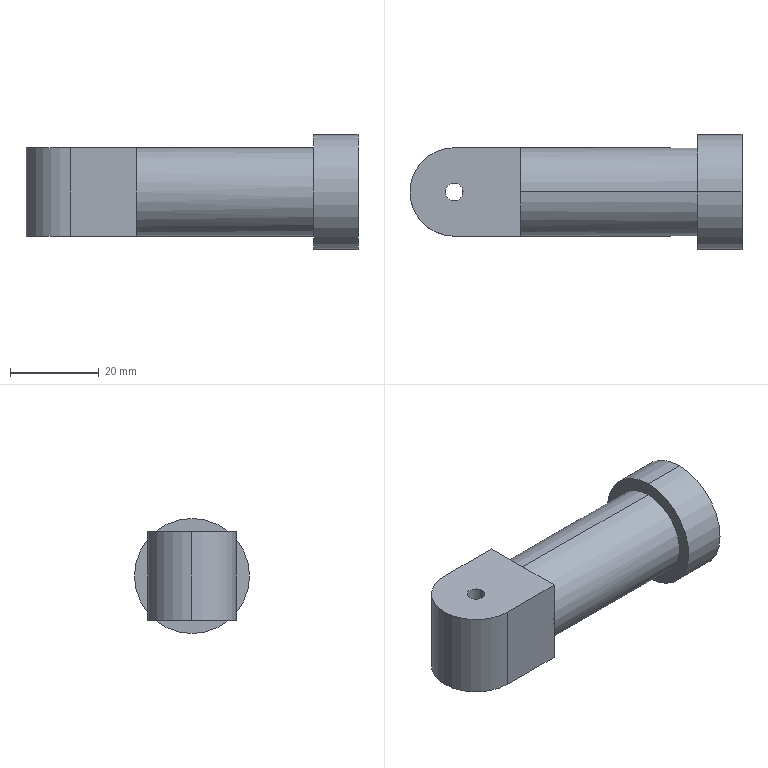Part | SolidWorks | features BaseBody 1 | 1 solid | 22 faces | box 75 x 26 x 26 mm | volume 24031 mm3 | cylinder 10 | plane 10 | cone 2 | commonest cylinder face diameters 20 x4 4 x2 16 x2 26 x2
STEP:
#1=CARTESIAN_POINT('',(15.081,-24.276,18.));
#2=VERTEX_POINT('',#1);
#3=CARTESIAN_POINT('',(15.081,-24.276,2.));
#4=VERTEX_POINT('',#3);
#5=CARTESIAN_POINT('',(15.081,-24.276,10.));
#6=DIRECTION('',(1.,0.,0.));
#7=DIRECTION('',(0.,0.,-1.));
#8=AXIS2_PLACEMENT_3D('',#5,#6,#7);
#9=CIRCLE('',#8,8.);
#10=EDGE_CURVE('',#2,#4,#9,.T.);
#11=ORIENTED_EDGE('',*,*,#10,.F.);
#12=CARTESIAN_POINT('',(27.081,-24.276,18.));
#13=VERTEX_POINT('',#12);
#14=CARTESIAN_POINT('',(27.081,-24.276,18.));
#15=DIRECTION('',(1.,0.,0.));
#16=VECTOR('',#15,1000.);
#17=LINE('',#14,#16);
#18=EDGE_CURVE('',#2,#13,#17,.T.);
#19=ORIENTED_EDGE('',*,*,#18,.T.);
#20=CARTESIAN_POINT('',(27.081,-24.276,2.));
#21=VERTEX_POINT('',#20);
#22=CARTESIAN_POINT('',(27.081,-24.276,10.));
#23=DIRECTION('',(1.,0.,0.));
#24=DIRECTION('',(0.,0.,-1.));
#25=AXIS2_PLACEMENT_3D('',#22,#23,#24);
#26=CIRCLE('',#25,8.);
#27=EDGE_CURVE('',#13,#21,#26,.T.);
#28=ORIENTED_EDGE('',*,*,#27,.T.);
#29=CARTESIAN_POINT('',(27.081,-24.276,2.));
#30=DIRECTION('',(1.,0.,0.));
#31=VECTOR('',#30,1000.);
#32=LINE('',#29,#31);
#33=EDGE_CURVE('',#4,#21,#32,.T.);
#34=ORIENTED_EDGE('',*,*,#33,.F.);
#35=EDGE_LOOP('',(#11,#19,#28,#34));
#36=FACE_OUTER_BOUND('',#35,.T.);
#37=CARTESIAN_POINT('',(27.081,-24.276,10.));
#38=DIRECTION('',(1.,0.,0.));
#39=DIRECTION('',(0.,0.,-1.));
#40=AXIS2_PLACEMENT_3D('',#37,#38,#39);
#41=CYLINDRICAL_SURFACE('',#40,8.);
#42=ADVANCED_FACE('',(#36),#41,.F.);
#43=CARTESIAN_POINT('',(10.274,-24.276,10.));
#44=VERTEX_POINT('',#43);
#45=CARTESIAN_POINT('',(15.081,-24.276,2.));
#46=DIRECTION('',(0.515,0.,-0.8572));
#47=VECTOR('',#46,1000.);
#48=LINE('',#45,#47);
#49=EDGE_CURVE('',#44,#4,#48,.T.);
#50=ORIENTED_EDGE('',*,*,#49,.F.);
#51=CARTESIAN_POINT('',(15.081,-24.276,18.));
#52=DIRECTION('',(0.515,0.,0.8572));
#53=VECTOR('',#52,1000.);
#54=LINE('',#51,#53);
#55=EDGE_CURVE('',#44,#2,#54,.T.);
#56=ORIENTED_EDGE('',*,*,#55,.T.);
#57=ORIENTED_EDGE('',*,*,#10,.T.);
#58=EDGE_LOOP('',(#50,#56,#57));
#59=FACE_OUTER_BOUND('',#58,.T.);
#60=CARTESIAN_POINT('',(15.081,-24.276,10.));
#61=DIRECTION('',(1.,0.,0.));
#62=DIRECTION('',(0.,0.,-1.));
#63=AXIS2_PLACEMENT_3D('',#60,#61,#62);
#64=CONICAL_SURFACE('',#63,8.,1.03);
#65=ADVANCED_FACE('',(#59),#64,.F.);
#66=CARTESIAN_POINT('',(17.081,-24.276,-3.));
#67=VERTEX_POINT('',#66);
#68=CARTESIAN_POINT('',(17.081,-24.276,23.));
#69=VERTEX_POINT('',#68);
#70=CARTESIAN_POINT('',(17.081,-24.276,10.));
#71=DIRECTION('',(1.,0.,0.));
#72=DIRECTION('',(0.,0.,-1.));
#73=AXIS2_PLACEMENT_3D('',#70,#71,#72);
#74=CIRCLE('',#73,13.);
#75=EDGE_CURVE('',#67,#69,#74,.T.);
#76=ORIENTED_EDGE('',*,*,#75,.T.);
#77=CARTESIAN_POINT('',(27.081,-24.276,23.));
#78=VERTEX_POINT('',#77);
#79=CARTESIAN_POINT('',(17.081,-24.276,23.));
#80=DIRECTION('',(1.,0.,0.));
#81=VECTOR('',#80,1000.);
#82=LINE('',#79,#81);
#83=EDGE_CURVE('',#69,#78,#82,.T.);
#84=ORIENTED_EDGE('',*,*,#83,.T.);
#85=CARTESIAN_POINT('',(27.081,-24.276,-3.));
#86=VERTEX_POINT('',#85);
#87=CARTESIAN_POINT('',(27.081,-24.276,10.));
#88=DIRECTION('',(1.,0.,0.));
#89=DIRECTION('',(0.,0.,-1.));
#90=AXIS2_PLACEMENT_3D('',#87,#88,#89);
#91=CIRCLE('',#90,13.);
#92=EDGE_CURVE('',#86,#78,#91,.T.);
#93=ORIENTED_EDGE('',*,*,#92,.F.);
#94=CARTESIAN_POINT('',(17.081,-24.276,-3.));
#95=DIRECTION('',(1.,0.,0.));
#96=VECTOR('',#95,1000.);
#97=LINE('',#94,#96);
#98=EDGE_CURVE('',#67,#86,#97,.T.);
#99=ORIENTED_EDGE('',*,*,#98,.F.);
#100=EDGE_LOOP('',(#76,#84,#93,#99));
#101=FACE_OUTER_BOUND('',#100,.T.);
#102=CARTESIAN_POINT('',(17.081,-24.276,10.));
#103=DIRECTION('',(1.,0.,0.));
#104=DIRECTION('',(0.,0.,-1.));
#105=AXIS2_PLACEMENT_3D('',#102,#103,#104);
#106=CYLINDRICAL_SURFACE('',#105,13.);
#107=ADVANCED_FACE('',(#101),#106,.T.);
#108=CARTESIAN_POINT('',(-39.919,-24.276,0.));
#109=VERTEX_POINT('',#108);
#110=CARTESIAN_POINT('',(-35.919,-24.276,0.));
#111=VERTEX_POINT('',#110);
#112=CARTESIAN_POINT('',(-37.919,-24.276,0.));
#113=DIRECTION('',(0.,0.,1.));
#114=DIRECTION('',(1.,0.,0.));
#115=AXIS2_PLACEMENT_3D('',#112,#113,#114);
#116=CIRCLE('',#115,2.);
#117=EDGE_CURVE('',#109,#111,#116,.T.);
#118=ORIENTED_EDGE('',*,*,#117,.F.);
#119=CARTESIAN_POINT('',(-39.919,-24.276,20.));
#120=VERTEX_POINT('',#119);
#121=CARTESIAN_POINT('',(-39.919,-24.276,20.));
#122=DIRECTION('',(0.,0.,1.));
#123=VECTOR('',#122,1000.);
#124=LINE('',#121,#123);
#125=EDGE_CURVE('',#109,#120,#124,.T.);
#126=ORIENTED_EDGE('',*,*,#125,.T.);
#127=CARTESIAN_POINT('',(-35.919,-24.276,20.));
#128=VERTEX_POINT('',#127);
#129=CARTESIAN_POINT('',(-37.919,-24.276,20.));
#130=DIRECTION('',(0.,0.,1.));
#131=DIRECTION('',(1.,0.,0.));
#132=AXIS2_PLACEMENT_3D('',#129,#130,#131);
#133=CIRCLE('',#132,2.);
#134=EDGE_CURVE('',#120,#128,#133,.T.);
#135=ORIENTED_EDGE('',*,*,#134,.T.);
#136=CARTESIAN_POINT('',(-35.919,-24.276,20.));
#137=DIRECTION('',(0.,0.,1.));
#138=VECTOR('',#137,1000.);
#139=LINE('',#136,#138);
#140=EDGE_CURVE('',#111,#128,#139,.T.);
#141=ORIENTED_EDGE('',*,*,#140,.F.);
#142=EDGE_LOOP('',(#118,#126,#135,#141));
#143=FACE_OUTER_BOUND('',#142,.T.);
#144=CARTESIAN_POINT('',(-37.919,-24.276,20.));
#145=DIRECTION('',(0.,0.,1.));
#146=DIRECTION('',(1.,0.,0.));
#147=AXIS2_PLACEMENT_3D('',#144,#145,#146);
#148=CYLINDRICAL_SURFACE('',#147,2.);
#149=ADVANCED_FACE('',(#143),#148,.F.);
#150=CARTESIAN_POINT('',(-47.919,-24.276,20.));
#151=VERTEX_POINT('',#150);
#152=CARTESIAN_POINT('',(-37.919,-34.276,20.));
#153=VERTEX_POINT('',#152);
#154=CARTESIAN_POINT('',(-37.919,-24.276,20.));
#155=DIRECTION('',(0.,0.,1.));
#156=DIRECTION('',(1.,0.,0.));
#157=AXIS2_PLACEMENT_3D('',#154,#155,#156);
#158=CIRCLE('',#157,10.);
#159=EDGE_CURVE('',#151,#153,#158,.T.);
#160=ORIENTED_EDGE('',*,*,#159,.F.);
#161=CARTESIAN_POINT('',(-47.919,-24.276,0.));
#162=VERTEX_POINT('',#161);
#163=CARTESIAN_POINT('',(-47.919,-24.276,20.));
#164=DIRECTION('',(0.,0.,-1.));
#165=VECTOR('',#164,1000.);
#166=LINE('',#163,#165);
#167=EDGE_CURVE('',#151,#162,#166,.T.);
#168=ORIENTED_EDGE('',*,*,#167,.T.);
#169=CARTESIAN_POINT('',(-37.919,-34.276,0.));
#170=VERTEX_POINT('',#169);
#171=CARTESIAN_POINT('',(-37.919,-24.276,0.));
#172=DIRECTION('',(0.,0.,1.));
#173=DIRECTION('',(1.,0.,0.));
#174=AXIS2_PLACEMENT_3D('',#171,#172,#173);
#175=CIRCLE('',#174,10.);
#176=EDGE_CURVE('',#162,#170,#175,.T.);
#177=ORIENTED_EDGE('',*,*,#176,.T.);
#178=CARTESIAN_POINT('',(-37.919,-34.276,20.));
#179=DIRECTION('',(0.,0.,-1.));
#180=VECTOR('',#179,1000.);
#181=LINE('',#178,#180);
#182=EDGE_CURVE('',#153,#170,#181,.T.);
#183=ORIENTED_EDGE('',*,*,#182,.F.);
#184=EDGE_LOOP('',(#160,#168,#177,#183));
#185=FACE_OUTER_BOUND('',#184,.T.);
#186=CARTESIAN_POINT('',(-37.919,-24.276,20.));
#187=DIRECTION('',(0.,0.,-1.));
#188=DIRECTION('',(-1.,0.,0.));
#189=AXIS2_PLACEMENT_3D('',#186,#187,#188);
#190=CYLINDRICAL_SURFACE('',#189,10.);
#191=ADVANCED_FACE('',(#185),#190,.T.);
#192=CARTESIAN_POINT('',(-22.919,-14.276,10.));
#193=VERTEX_POINT('',#192);
#194=CARTESIAN_POINT('',(-22.919,-24.276,20.));
#195=VERTEX_POINT('',#194);
#196=CARTESIAN_POINT('',(-22.919,-24.276,10.));
#197=DIRECTION('',(1.,0.,0.));
#198=DIRECTION('',(0.,0.,-1.));
#199=AXIS2_PLACEMENT_3D('',#196,#197,#198);
#200=CIRCLE('',#199,10.);
#201=EDGE_CURVE('',#193,#195,#200,.T.);
#202=ORIENTED_EDGE('',*,*,#201,.T.);
#203=CARTESIAN_POINT('',(17.081,-24.276,20.));
#204=VERTEX_POINT('',#203);
#205=CARTESIAN_POINT('',(-22.919,-24.276,20.));
#206=DIRECTION('',(1.,0.,0.));
#207=VECTOR('',#206,1000.);
#208=LINE('',#205,#207);
#209=EDGE_CURVE('',#195,#204,#208,.T.);
#210=ORIENTED_EDGE('',*,*,#209,.T.);
#211=CARTESIAN_POINT('',(17.081,-24.276,0.));
#212=VERTEX_POINT('',#211);
#213=CARTESIAN_POINT('',(17.081,-24.276,10.));
#214=DIRECTION('',(-1.,0.,0.));
#215=DIRECTION('',(0.,0.,-1.));
#216=AXIS2_PLACEMENT_3D('',#213,#214,#215);
#217=CIRCLE('',#216,10.);
#218=EDGE_CURVE('',#204,#212,#217,.T.);
#219=ORIENTED_EDGE('',*,*,#218,.T.);
#220=CARTESIAN_POINT('',(-22.919,-24.276,0.));
#221=VERTEX_POINT('',#220);
#222=CARTESIAN_POINT('',(-22.919,-24.276,0.));
#223=DIRECTION('',(1.,0.,0.));
#224=VECTOR('',#223,1000.);
#225=LINE('',#222,#224);
#226=EDGE_CURVE('',#221,#212,#225,.T.);
#227=ORIENTED_EDGE('',*,*,#226,.F.);
#228=CARTESIAN_POINT('',(-22.919,-24.276,10.));
#229=DIRECTION('',(1.,0.,0.));
#230=DIRECTION('',(0.,0.,-1.));
#231=AXIS2_PLACEMENT_3D('',#228,#229,#230);
#232=CIRCLE('',#231,10.);
#233=EDGE_CURVE('',#221,#193,#232,.T.);
#234=ORIENTED_EDGE('',*,*,#233,.T.);
#235=EDGE_LOOP('',(#202,#210,#219,#227,#234));
#236=FACE_OUTER_BOUND('',#235,.T.);
#237=CARTESIAN_POINT('',(-22.919,-24.276,10.));
#238=DIRECTION('',(1.,0.,0.));
#239=DIRECTION('',(0.,0.,-1.));
#240=AXIS2_PLACEMENT_3D('',#237,#238,#239);
#241=CYLINDRICAL_SURFACE('',#240,10.);
#242=ADVANCED_FACE('',(#236),#241,.T.);
#243=CARTESIAN_POINT('',(27.081,-24.276,10.));
#244=DIRECTION('',(1.,0.,0.));
#245=DIRECTION('',(0.,0.,-1.));
#246=AXIS2_PLACEMENT_3D('',#243,#244,#245);
#247=CIRCLE('',#246,8.);
#248=EDGE_CURVE('',#21,#13,#247,.T.);
#249=ORIENTED_EDGE('',*,*,#248,.F.);
#250=ORIENTED_EDGE('',*,*,#27,.F.);
#251=EDGE_LOOP('',(#249,#250));
#252=FACE_BOUND('',#251,.T.);
#253=ORIENTED_EDGE('',*,*,#92,.T.);
#254=CARTESIAN_POINT('',(27.081,-24.276,10.));
#255=DIRECTION('',(1.,0.,0.));
#256=DIRECTION('',(0.,0.,-1.));
#257=AXIS2_PLACEMENT_3D('',#254,#255,#256);
#258=CIRCLE('',#257,13.);
#259=EDGE_CURVE('',#78,#86,#258,.T.);
#260=ORIENTED_EDGE('',*,*,#259,.T.);
#261=EDGE_LOOP('',(#253,#260));
#262=FACE_OUTER_BOUND('',#261,.T.);
#263=CARTESIAN_POINT('',(27.081,-14.276,20.));
#264=DIRECTION('',(-1.,0.,0.));
#265=DIRECTION('',(0.,0.,1.));
#266=AXIS2_PLACEMENT_3D('',#263,#264,#265);
#267=PLANE('',#266);
#268=ADVANCED_FACE('',(#252,#262),#267,.F.);
#269=CARTESIAN_POINT('',(17.081,-24.276,10.));
#270=DIRECTION('',(-1.,0.,0.));
#271=DIRECTION('',(0.,0.,-1.));
#272=AXIS2_PLACEMENT_3D('',#269,#270,#271);
#273=CIRCLE('',#272,10.);
#274=EDGE_CURVE('',#212,#204,#273,.T.);
#275=ORIENTED_EDGE('',*,*,#274,.F.);
#276=ORIENTED_EDGE('',*,*,#218,.F.);
#277=EDGE_LOOP('',(#275,#276));
#278=FACE_BOUND('',#277,.T.);
#279=ORIENTED_EDGE('',*,*,#75,.F.);
#280=CARTESIAN_POINT('',(17.081,-24.276,10.));
#281=DIRECTION('',(1.,0.,0.));
#282=DIRECTION('',(0.,0.,-1.));
#283=AXIS2_PLACEMENT_3D('',#280,#281,#282);
#284=CIRCLE('',#283,13.);
#285=EDGE_CURVE('',#69,#67,#284,.T.);
#286=ORIENTED_EDGE('',*,*,#285,.F.);
#287=EDGE_LOOP('',(#279,#286));
#288=FACE_OUTER_BOUND('',#287,.T.);
#289=CARTESIAN_POINT('',(17.081,-24.276,10.));
#290=DIRECTION('',(1.,0.,0.));
#291=DIRECTION('',(0.,1.,0.));
#292=AXIS2_PLACEMENT_3D('',#289,#290,#291);
#293=PLANE('',#292);
#294=ADVANCED_FACE('',(#278,#288),#293,.F.);
#295=CARTESIAN_POINT('',(-22.919,-34.276,20.));
#296=VERTEX_POINT('',#295);
#297=CARTESIAN_POINT('',(-22.919,-34.276,10.));
#298=VERTEX_POINT('',#297);
#299=CARTESIAN_POINT('',(-22.919,-34.276,20.));
#300=DIRECTION('',(0.,0.,-1.));
#301=VECTOR('',#300,1000.);
#302=LINE('',#299,#301);
#303=EDGE_CURVE('',#296,#298,#302,.T.);
#304=ORIENTED_EDGE('',*,*,#303,.T.);
#305=CARTESIAN_POINT('',(-22.919,-24.276,10.));
#306=DIRECTION('',(1.,0.,0.));
#307=DIRECTION('',(0.,0.,-1.));
#308=AXIS2_PLACEMENT_3D('',#305,#306,#307);
#309=CIRCLE('',#308,10.);
#310=EDGE_CURVE('',#195,#298,#309,.T.);
#311=ORIENTED_EDGE('',*,*,#310,.F.);
#312=CARTESIAN_POINT('',(-22.919,-24.276,20.));
#313=DIRECTION('',(0.,1.,0.));
#314=VECTOR('',#313,1000.);
#315=LINE('',#312,#314);
#316=EDGE_CURVE('',#296,#195,#315,.T.);
#317=ORIENTED_EDGE('',*,*,#316,.F.);
#318=EDGE_LOOP('',(#304,#311,#317));
#319=FACE_OUTER_BOUND('',#318,.T.);
#320=CARTESIAN_POINT('',(-22.919,-24.276,10.));
#321=DIRECTION('',(1.,0.,0.));
#322=DIRECTION('',(0.,1.,0.));
#323=AXIS2_PLACEMENT_3D('',#320,#321,#322);
#324=PLANE('',#323);
#325=ADVANCED_FACE('',(#319),#324,.T.);
#326=CARTESIAN_POINT('',(-22.919,-14.276,0.));
#327=VERTEX_POINT('',#326);
#328=CARTESIAN_POINT('',(-22.919,-14.276,20.));
#329=DIRECTION('',(0.,0.,1.));
#330=VECTOR('',#329,1000.);
#331=LINE('',#328,#330);
#332=EDGE_CURVE('',#327,#193,#331,.T.);
#333=ORIENTED_EDGE('',*,*,#332,.T.);
#334=ORIENTED_EDGE('',*,*,#233,.F.);
#335=CARTESIAN_POINT('',(-22.919,-24.276,0.));
#336=DIRECTION('',(0.,1.,0.));
#337=VECTOR('',#336,1000.);
#338=LINE('',#335,#337);
#339=EDGE_CURVE('',#221,#327,#338,.T.);
#340=ORIENTED_EDGE('',*,*,#339,.T.);
#341=EDGE_LOOP('',(#333,#334,#340));
#342=FACE_OUTER_BOUND('',#341,.T.);
#343=CARTESIAN_POINT('',(-22.919,-24.276,10.));
#344=DIRECTION('',(1.,0.,0.));
#345=DIRECTION('',(0.,1.,0.));
#346=AXIS2_PLACEMENT_3D('',#343,#344,#345);
#347=PLANE('',#346);
#348=ADVANCED_FACE('',(#342),#347,.T.);
#349=CARTESIAN_POINT('',(-22.919,-34.276,0.));
#350=VERTEX_POINT('',#349);
#351=CARTESIAN_POINT('',(-22.919,-34.276,20.));
#352=DIRECTION('',(0.,0.,-1.));
#353=VECTOR('',#352,1000.);
#354=LINE('',#351,#353);
#355=EDGE_CURVE('',#298,#350,#354,.T.);
#356=ORIENTED_EDGE('',*,*,#355,.T.);
#357=CARTESIAN_POINT('',(-22.919,-24.276,0.));
#358=DIRECTION('',(0.,1.,0.));
#359=VECTOR('',#358,1000.);
#360=LINE('',#357,#359);
#361=EDGE_CURVE('',#350,#221,#360,.T.);
#362=ORIENTED_EDGE('',*,*,#361,.T.);
#363=CARTESIAN_POINT('',(-22.919,-24.276,10.));
#364=DIRECTION('',(1.,0.,0.));
#365=DIRECTION('',(0.,0.,-1.));
#366=AXIS2_PLACEMENT_3D('',#363,#364,#365);
#367=CIRCLE('',#366,10.);
#368=EDGE_CURVE('',#298,#221,#367,.T.);
#369=ORIENTED_EDGE('',*,*,#368,.F.);
#370=EDGE_LOOP('',(#356,#362,#369));
#371=FACE_OUTER_BOUND('',#370,.T.);
#372=CARTESIAN_POINT('',(-22.919,-24.276,10.));
#373=DIRECTION('',(1.,0.,0.));
#374=DIRECTION('',(0.,1.,0.));
#375=AXIS2_PLACEMENT_3D('',#372,#373,#374);
#376=PLANE('',#375);
#377=ADVANCED_FACE('',(#371),#376,.T.);
#378=ORIENTED_EDGE('',*,*,#201,.F.);
#379=CARTESIAN_POINT('',(-22.919,-14.276,20.));
#380=VERTEX_POINT('',#379);
#381=CARTESIAN_POINT('',(-22.919,-14.276,20.));
#382=DIRECTION('',(0.,0.,1.));
#383=VECTOR('',#382,1000.);
#384=LINE('',#381,#383);
#385=EDGE_CURVE('',#193,#380,#384,.T.);
#386=ORIENTED_EDGE('',*,*,#385,.T.);
#387=CARTESIAN_POINT('',(-22.919,-24.276,20.));
#388=DIRECTION('',(0.,1.,0.));
#389=VECTOR('',#388,1000.);
#390=LINE('',#387,#389);
#391=EDGE_CURVE('',#195,#380,#390,.T.);
#392=ORIENTED_EDGE('',*,*,#391,.F.);
#393=EDGE_LOOP('',(#378,#386,#392));
#394=FACE_OUTER_BOUND('',#393,.T.);
#395=CARTESIAN_POINT('',(-22.919,-24.276,10.));
#396=DIRECTION('',(1.,0.,0.));
#397=DIRECTION('',(0.,1.,0.));
#398=AXIS2_PLACEMENT_3D('',#395,#396,#397);
#399=PLANE('',#398);
#400=ADVANCED_FACE('',(#394),#399,.T.);
#401=CARTESIAN_POINT('',(-37.919,-24.276,0.));
#402=DIRECTION('',(0.,0.,1.));
#403=DIRECTION('',(1.,0.,0.));
#404=AXIS2_PLACEMENT_3D('',#401,#402,#403);
#405=CIRCLE('',#404,2.);
#406=EDGE_CURVE('',#111,#109,#405,.T.);
#407=ORIENTED_EDGE('',*,*,#406,.T.);
#408=ORIENTED_EDGE('',*,*,#117,.T.);
#409=EDGE_LOOP('',(#407,#408));
#410=FACE_BOUND('',#409,.T.);
#411=ORIENTED_EDGE('',*,*,#361,.F.);
#412=CARTESIAN_POINT('',(-37.919,-34.276,0.));
#413=DIRECTION('',(1.,0.,0.));
#414=VECTOR('',#413,1000.);
#415=LINE('',#412,#414);
#416=EDGE_CURVE('',#170,#350,#415,.T.);
#417=ORIENTED_EDGE('',*,*,#416,.F.);
#418=ORIENTED_EDGE('',*,*,#176,.F.);
#419=CARTESIAN_POINT('',(-37.919,-14.276,0.));
#420=VERTEX_POINT('',#419);
#421=CARTESIAN_POINT('',(-37.919,-24.276,0.));
#422=DIRECTION('',(0.,0.,1.));
#423=DIRECTION('',(1.,0.,0.));
#424=AXIS2_PLACEMENT_3D('',#421,#422,#423);
#425=CIRCLE('',#424,10.);
#426=EDGE_CURVE('',#420,#162,#425,.T.);
#427=ORIENTED_EDGE('',*,*,#426,.F.);
#428=CARTESIAN_POINT('',(-37.919,-14.276,0.));
#429=DIRECTION('',(-1.,0.,0.));
#430=VECTOR('',#429,1000.);
#431=LINE('',#428,#430);
#432=EDGE_CURVE('',#327,#420,#431,.T.);
#433=ORIENTED_EDGE('',*,*,#432,.F.);
#434=ORIENTED_EDGE('',*,*,#339,.F.);
#435=EDGE_LOOP('',(#411,#417,#418,#427,#433,#434));
#436=FACE_OUTER_BOUND('',#435,.T.);
#437=CARTESIAN_POINT('',(-37.919,-24.276,0.));
#438=DIRECTION('',(0.,0.,1.));
#439=DIRECTION('',(1.,0.,0.));
#440=AXIS2_PLACEMENT_3D('',#437,#438,#439);
#441=PLANE('',#440);
#442=ADVANCED_FACE('',(#410,#436),#441,.F.);
#443=CARTESIAN_POINT('',(-37.919,-24.276,20.));
#444=DIRECTION('',(0.,0.,1.));
#445=DIRECTION('',(1.,0.,0.));
#446=AXIS2_PLACEMENT_3D('',#443,#444,#445);
#447=CIRCLE('',#446,2.);
#448=EDGE_CURVE('',#128,#120,#447,.T.);
#449=ORIENTED_EDGE('',*,*,#448,.F.);
#450=ORIENTED_EDGE('',*,*,#134,.F.);
#451=EDGE_LOOP('',(#449,#450));
#452=FACE_BOUND('',#451,.T.);
#453=CARTESIAN_POINT('',(-37.919,-34.276,20.));
#454=DIRECTION('',(1.,0.,0.));
#455=VECTOR('',#454,1000.);
#456=LINE('',#453,#455);
#457=EDGE_CURVE('',#153,#296,#456,.T.);
#458=ORIENTED_EDGE('',*,*,#457,.T.);
#459=ORIENTED_EDGE('',*,*,#316,.T.);
#460=ORIENTED_EDGE('',*,*,#391,.T.);
#461=CARTESIAN_POINT('',(-37.919,-14.276,20.));
#462=VERTEX_POINT('',#461);
#463=CARTESIAN_POINT('',(-37.919,-14.276,20.));
#464=DIRECTION('',(-1.,0.,0.));
#465=VECTOR('',#464,1000.);
#466=LINE('',#463,#465);
#467=EDGE_CURVE('',#380,#462,#466,.T.);
#468=ORIENTED_EDGE('',*,*,#467,.T.);
#469=CARTESIAN_POINT('',(-37.919,-24.276,20.));
#470=DIRECTION('',(0.,0.,1.));
#471=DIRECTION('',(1.,0.,0.));
#472=AXIS2_PLACEMENT_3D('',#469,#470,#471);
#473=CIRCLE('',#472,10.);
#474=EDGE_CURVE('',#462,#151,#473,.T.);
#475=ORIENTED_EDGE('',*,*,#474,.T.);
#476=ORIENTED_EDGE('',*,*,#159,.T.);
#477=EDGE_LOOP('',(#458,#459,#460,#468,#475,#476));
#478=FACE_OUTER_BOUND('',#477,.T.);
#479=CARTESIAN_POINT('',(-37.919,-24.276,20.));
#480=DIRECTION('',(0.,0.,1.));
#481=DIRECTION('',(1.,0.,0.));
#482=AXIS2_PLACEMENT_3D('',#479,#480,#481);
#483=PLANE('',#482);
#484=ADVANCED_FACE('',(#452,#478),#483,.T.);
#485=ORIENTED_EDGE('',*,*,#332,.F.);
#486=ORIENTED_EDGE('',*,*,#432,.T.);
#487=CARTESIAN_POINT('',(-37.919,-14.276,20.));
#488=DIRECTION('',(0.,0.,-1.));
#489=VECTOR('',#488,1000.);
#490=LINE('',#487,#489);
#491=EDGE_CURVE('',#462,#420,#490,.T.);
#492=ORIENTED_EDGE('',*,*,#491,.F.);
#493=ORIENTED_EDGE('',*,*,#467,.F.);
#494=ORIENTED_EDGE('',*,*,#385,.F.);
#495=EDGE_LOOP('',(#485,#486,#492,#493,#494));
#496=FACE_OUTER_BOUND('',#495,.T.);
#497=CARTESIAN_POINT('',(-37.919,-14.276,20.));
#498=DIRECTION('',(0.,-1.,0.));
#499=DIRECTION('',(0.,0.,-1.));
#500=AXIS2_PLACEMENT_3D('',#497,#498,#499);
#501=PLANE('',#500);
#502=ADVANCED_FACE('',(#496),#501,.F.);
#503=ORIENTED_EDGE('',*,*,#303,.F.);
#504=ORIENTED_EDGE('',*,*,#457,.F.);
#505=ORIENTED_EDGE('',*,*,#182,.T.);
#506=ORIENTED_EDGE('',*,*,#416,.T.);
#507=ORIENTED_EDGE('',*,*,#355,.F.);
#508=EDGE_LOOP('',(#503,#504,#505,#506,#507));
#509=FACE_OUTER_BOUND('',#508,.T.);
#510=CARTESIAN_POINT('',(-37.919,-34.276,20.));
#511=DIRECTION('',(0.,1.,0.));
#512=DIRECTION('',(1.,0.,0.));
#513=AXIS2_PLACEMENT_3D('',#510,#511,#512);
#514=PLANE('',#513);
#515=ADVANCED_FACE('',(#509),#514,.F.);
#516=ORIENTED_EDGE('',*,*,#209,.F.);
#517=ORIENTED_EDGE('',*,*,#310,.T.);
#518=ORIENTED_EDGE('',*,*,#368,.T.);
#519=ORIENTED_EDGE('',*,*,#226,.T.);
#520=ORIENTED_EDGE('',*,*,#274,.T.);
#521=EDGE_LOOP('',(#516,#517,#518,#519,#520));
#522=FACE_OUTER_BOUND('',#521,.T.);
#523=CARTESIAN_POINT('',(-22.919,-24.276,10.));
#524=DIRECTION('',(1.,0.,0.));
#525=DIRECTION('',(0.,0.,-1.));
#526=AXIS2_PLACEMENT_3D('',#523,#524,#525);
#527=CYLINDRICAL_SURFACE('',#526,10.);
#528=ADVANCED_FACE('',(#522),#527,.T.);
#529=ORIENTED_EDGE('',*,*,#167,.F.);
#530=ORIENTED_EDGE('',*,*,#474,.F.);
#531=ORIENTED_EDGE('',*,*,#491,.T.);
#532=ORIENTED_EDGE('',*,*,#426,.T.);
#533=EDGE_LOOP('',(#529,#530,#531,#532));
#534=FACE_OUTER_BOUND('',#533,.T.);
#535=CARTESIAN_POINT('',(-37.919,-24.276,20.));
#536=DIRECTION('',(0.,0.,-1.));
#537=DIRECTION('',(-1.,0.,0.));
#538=AXIS2_PLACEMENT_3D('',#535,#536,#537);
#539=CYLINDRICAL_SURFACE('',#538,10.);
#540=ADVANCED_FACE('',(#534),#539,.T.);
#541=ORIENTED_EDGE('',*,*,#125,.F.);
#542=ORIENTED_EDGE('',*,*,#406,.F.);
#543=ORIENTED_EDGE('',*,*,#140,.T.);
#544=ORIENTED_EDGE('',*,*,#448,.T.);
#545=EDGE_LOOP('',(#541,#542,#543,#544));
#546=FACE_OUTER_BOUND('',#545,.T.);
#547=CARTESIAN_POINT('',(-37.919,-24.276,20.));
#548=DIRECTION('',(0.,0.,1.));
#549=DIRECTION('',(1.,0.,0.));
#550=AXIS2_PLACEMENT_3D('',#547,#548,#549);
#551=CYLINDRICAL_SURFACE('',#550,2.);
#552=ADVANCED_FACE('',(#546),#551,.F.);
#553=ORIENTED_EDGE('',*,*,#83,.F.);
#554=ORIENTED_EDGE('',*,*,#285,.T.);
#555=ORIENTED_EDGE('',*,*,#98,.T.);
#556=ORIENTED_EDGE('',*,*,#259,.F.);
#557=EDGE_LOOP('',(#553,#554,#555,#556));
#558=FACE_OUTER_BOUND('',#557,.T.);
#559=CARTESIAN_POINT('',(17.081,-24.276,10.));
#560=DIRECTION('',(1.,0.,0.));
#561=DIRECTION('',(0.,0.,-1.));
#562=AXIS2_PLACEMENT_3D('',#559,#560,#561);
#563=CYLINDRICAL_SURFACE('',#562,13.);
#564=ADVANCED_FACE('',(#558),#563,.T.);
#565=ORIENTED_EDGE('',*,*,#55,.F.);
#566=ORIENTED_EDGE('',*,*,#49,.T.);
#567=CARTESIAN_POINT('',(15.081,-24.276,10.));
#568=DIRECTION('',(1.,0.,0.));
#569=DIRECTION('',(0.,0.,-1.));
#570=AXIS2_PLACEMENT_3D('',#567,#568,#569);
#571=CIRCLE('',#570,8.);
#572=EDGE_CURVE('',#4,#2,#571,.T.);
#573=ORIENTED_EDGE('',*,*,#572,.T.);
#574=EDGE_LOOP('',(#565,#566,#573));
#575=FACE_OUTER_BOUND('',#574,.T.);
#576=CARTESIAN_POINT('',(15.081,-24.276,10.));
#577=DIRECTION('',(1.,0.,0.));
#578=DIRECTION('',(0.,0.,-1.));
#579=AXIS2_PLACEMENT_3D('',#576,#577,#578);
#580=CONICAL_SURFACE('',#579,8.,1.03);
#581=ADVANCED_FACE('',(#575),#580,.F.);
#582=ORIENTED_EDGE('',*,*,#18,.F.);
#583=ORIENTED_EDGE('',*,*,#572,.F.);
#584=ORIENTED_EDGE('',*,*,#33,.T.);
#585=ORIENTED_EDGE('',*,*,#248,.T.);
#586=EDGE_LOOP('',(#582,#583,#584,#585));
#587=FACE_OUTER_BOUND('',#586,.T.);
#588=CARTESIAN_POINT('',(27.081,-24.276,10.));
#589=DIRECTION('',(1.,0.,0.));
#590=DIRECTION('',(0.,0.,-1.));
#591=AXIS2_PLACEMENT_3D('',#588,#589,#590);
#592=CYLINDRICAL_SURFACE('',#591,8.);
#593=ADVANCED_FACE('',(#587),#592,.F.);
#594=CLOSED_SHELL('',(#42,#65,#107,#149,#191,#242,#268,#294,#325,#348,#377,#400,#442,#484,#502,#515,#528,#540,#552,#564,#581,#593));
#595=MANIFOLD_SOLID_BREP('',#594);
#596=CARTESIAN_POINT('',(0.,0.,0.));
#597=DIRECTION('',(0.,0.,1.));
#598=DIRECTION('',(1.,0.,0.));
#599=AXIS2_PLACEMENT_3D('',#596,#597,#598);
#600=(LENGTH_UNIT()NAMED_UNIT(*)SI_UNIT(.MILLI.,.METRE.));
#601=UNCERTAINTY_MEASURE_WITH_UNIT(LENGTH_MEASURE(0.00001),#600,'','');
#602=(NAMED_UNIT(*)PLANE_ANGLE_UNIT()SI_UNIT($,.RADIAN.));
#603=(NAMED_UNIT(*)SI_UNIT($,.STERADIAN.)SOLID_ANGLE_UNIT());
#604=(GEOMETRIC_REPRESENTATION_CONTEXT(3)GLOBAL_UNCERTAINTY_ASSIGNED_CONTEXT((#601))GLOBAL_UNIT_ASSIGNED_CONTEXT((#600,#602,#603))REPRESENTATION_CONTEXT('',''));
#605=ADVANCED_BREP_SHAPE_REPRESENTATION('',(#595,#599),#604);